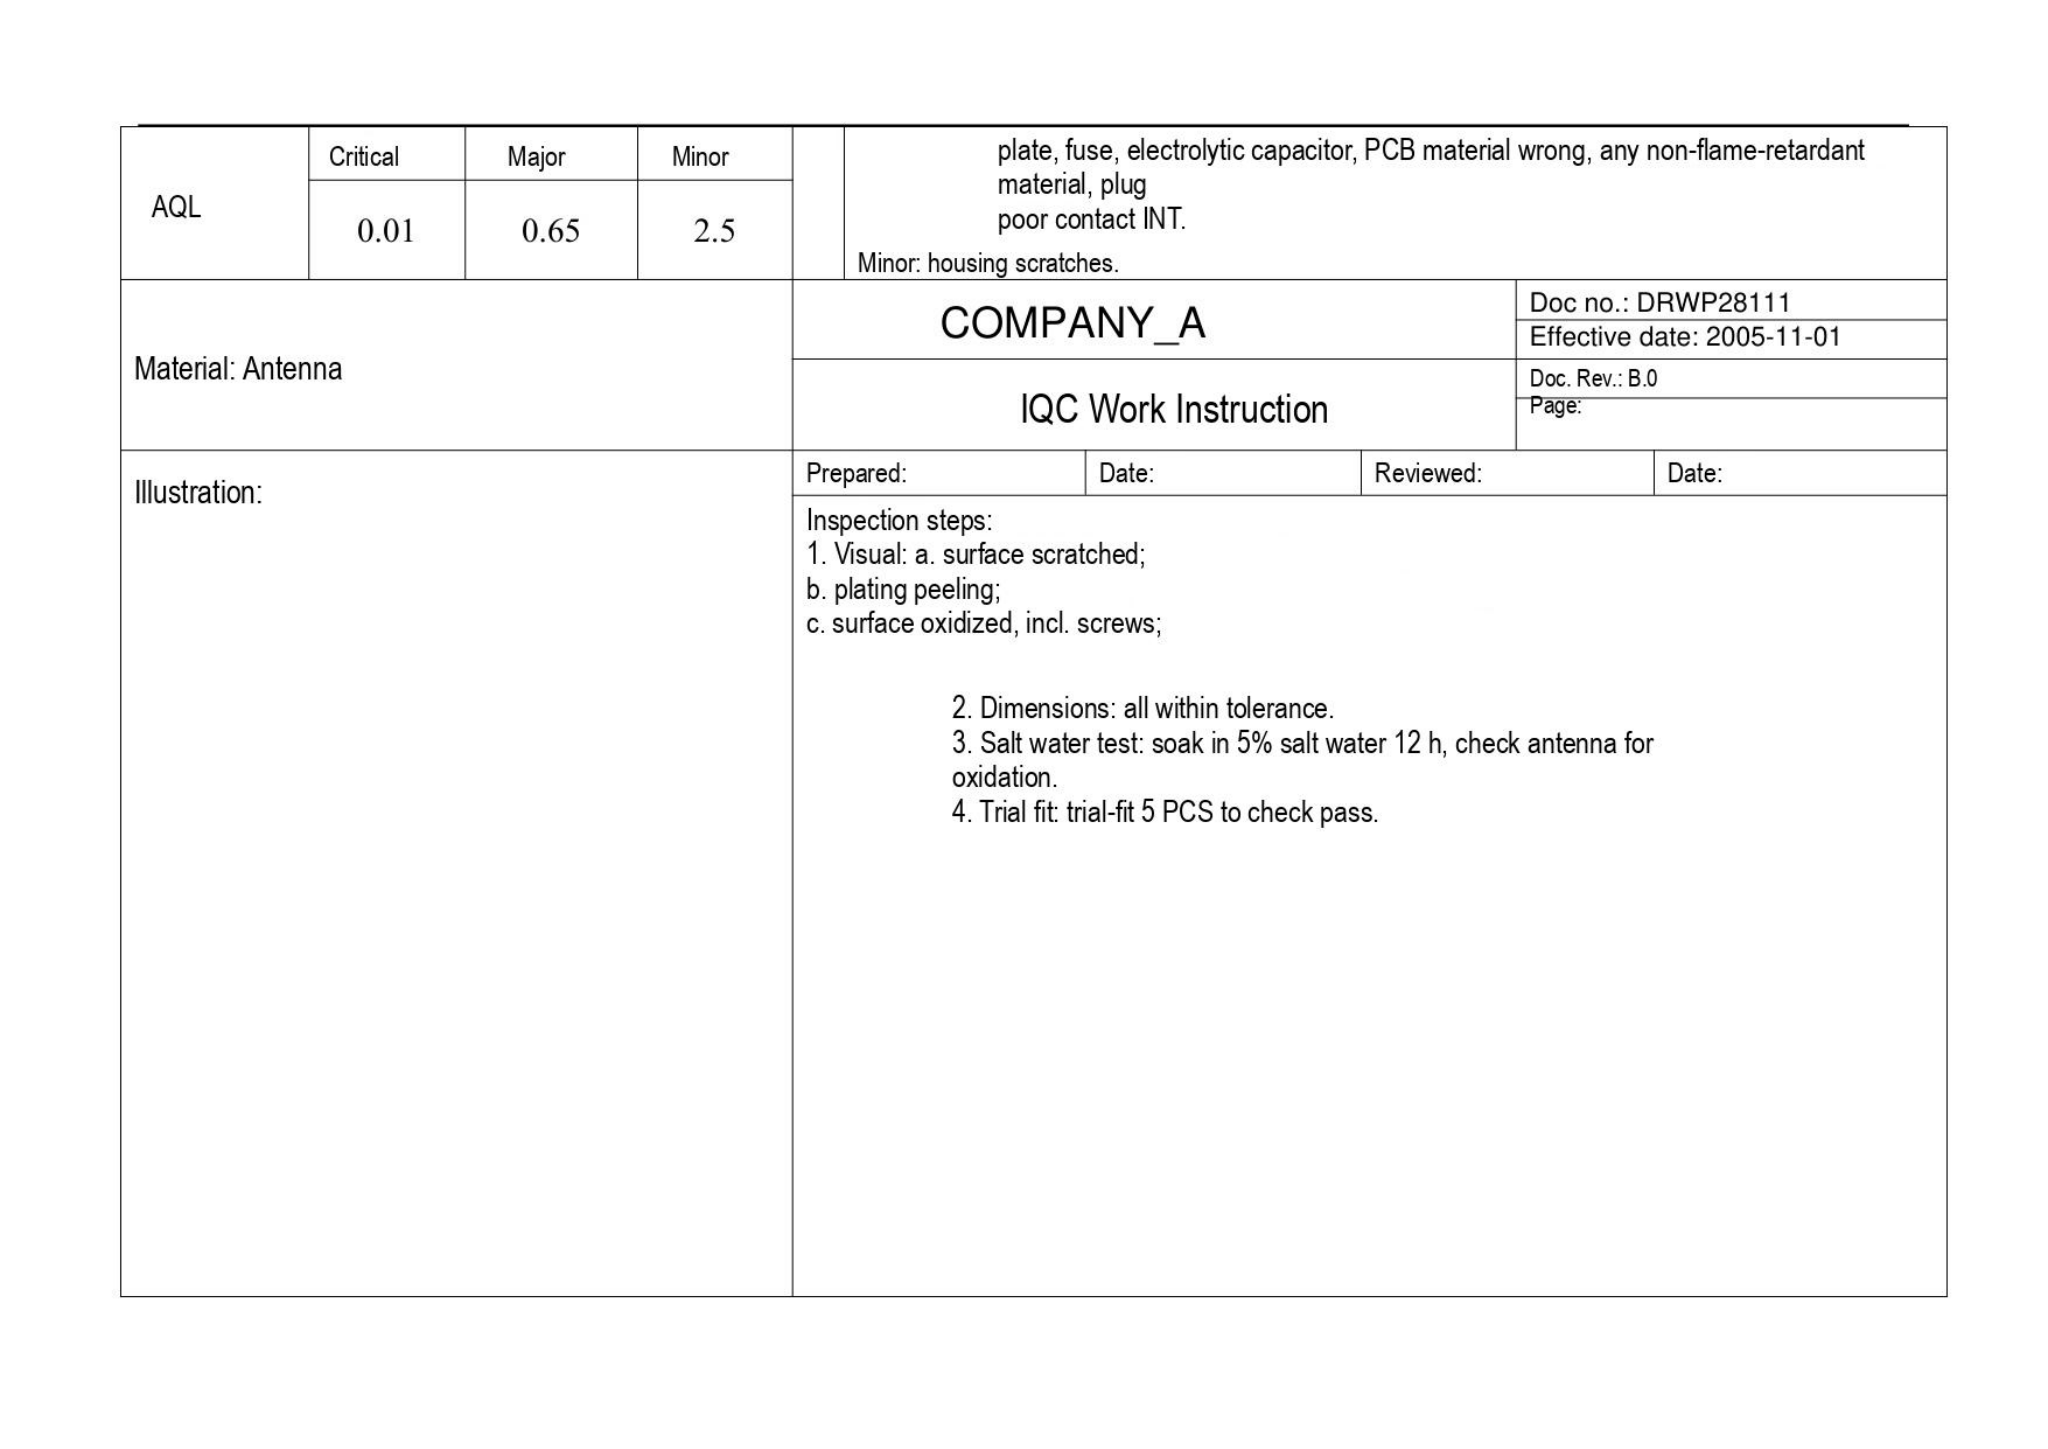| AQL | Critical | Major | Minor |
|---|---|---|---|
| | 0.01 | 0.65 | 2.5 |

plate, fuse, electrolytic capacitor, PCB material wrong, any non-flame-retardant material, plug
poor contact INT.
Minor: housing scratches.

Material: Antenna

| COMPANY_A | Doc no.: DRWP28111 |
|---|---|
| | Effective date: 2005-11-01 |
| IQC Work Instruction | Doc. Rev.: B.0 |
| | Page: |

Illustration:

| Prepared: | Date: | Reviewed: | Date: |
|---|---|---|---|

Inspection steps:
1. Visual: a. surface scratched;
b. plating peeling;
c. surface oxidized, incl. screws;

2. Dimensions: all within tolerance.
3. Salt water test: soak in 5% salt water 12 h, check antenna for oxidation.
4. Trial fit: trial-fit 5 PCS to check pass.
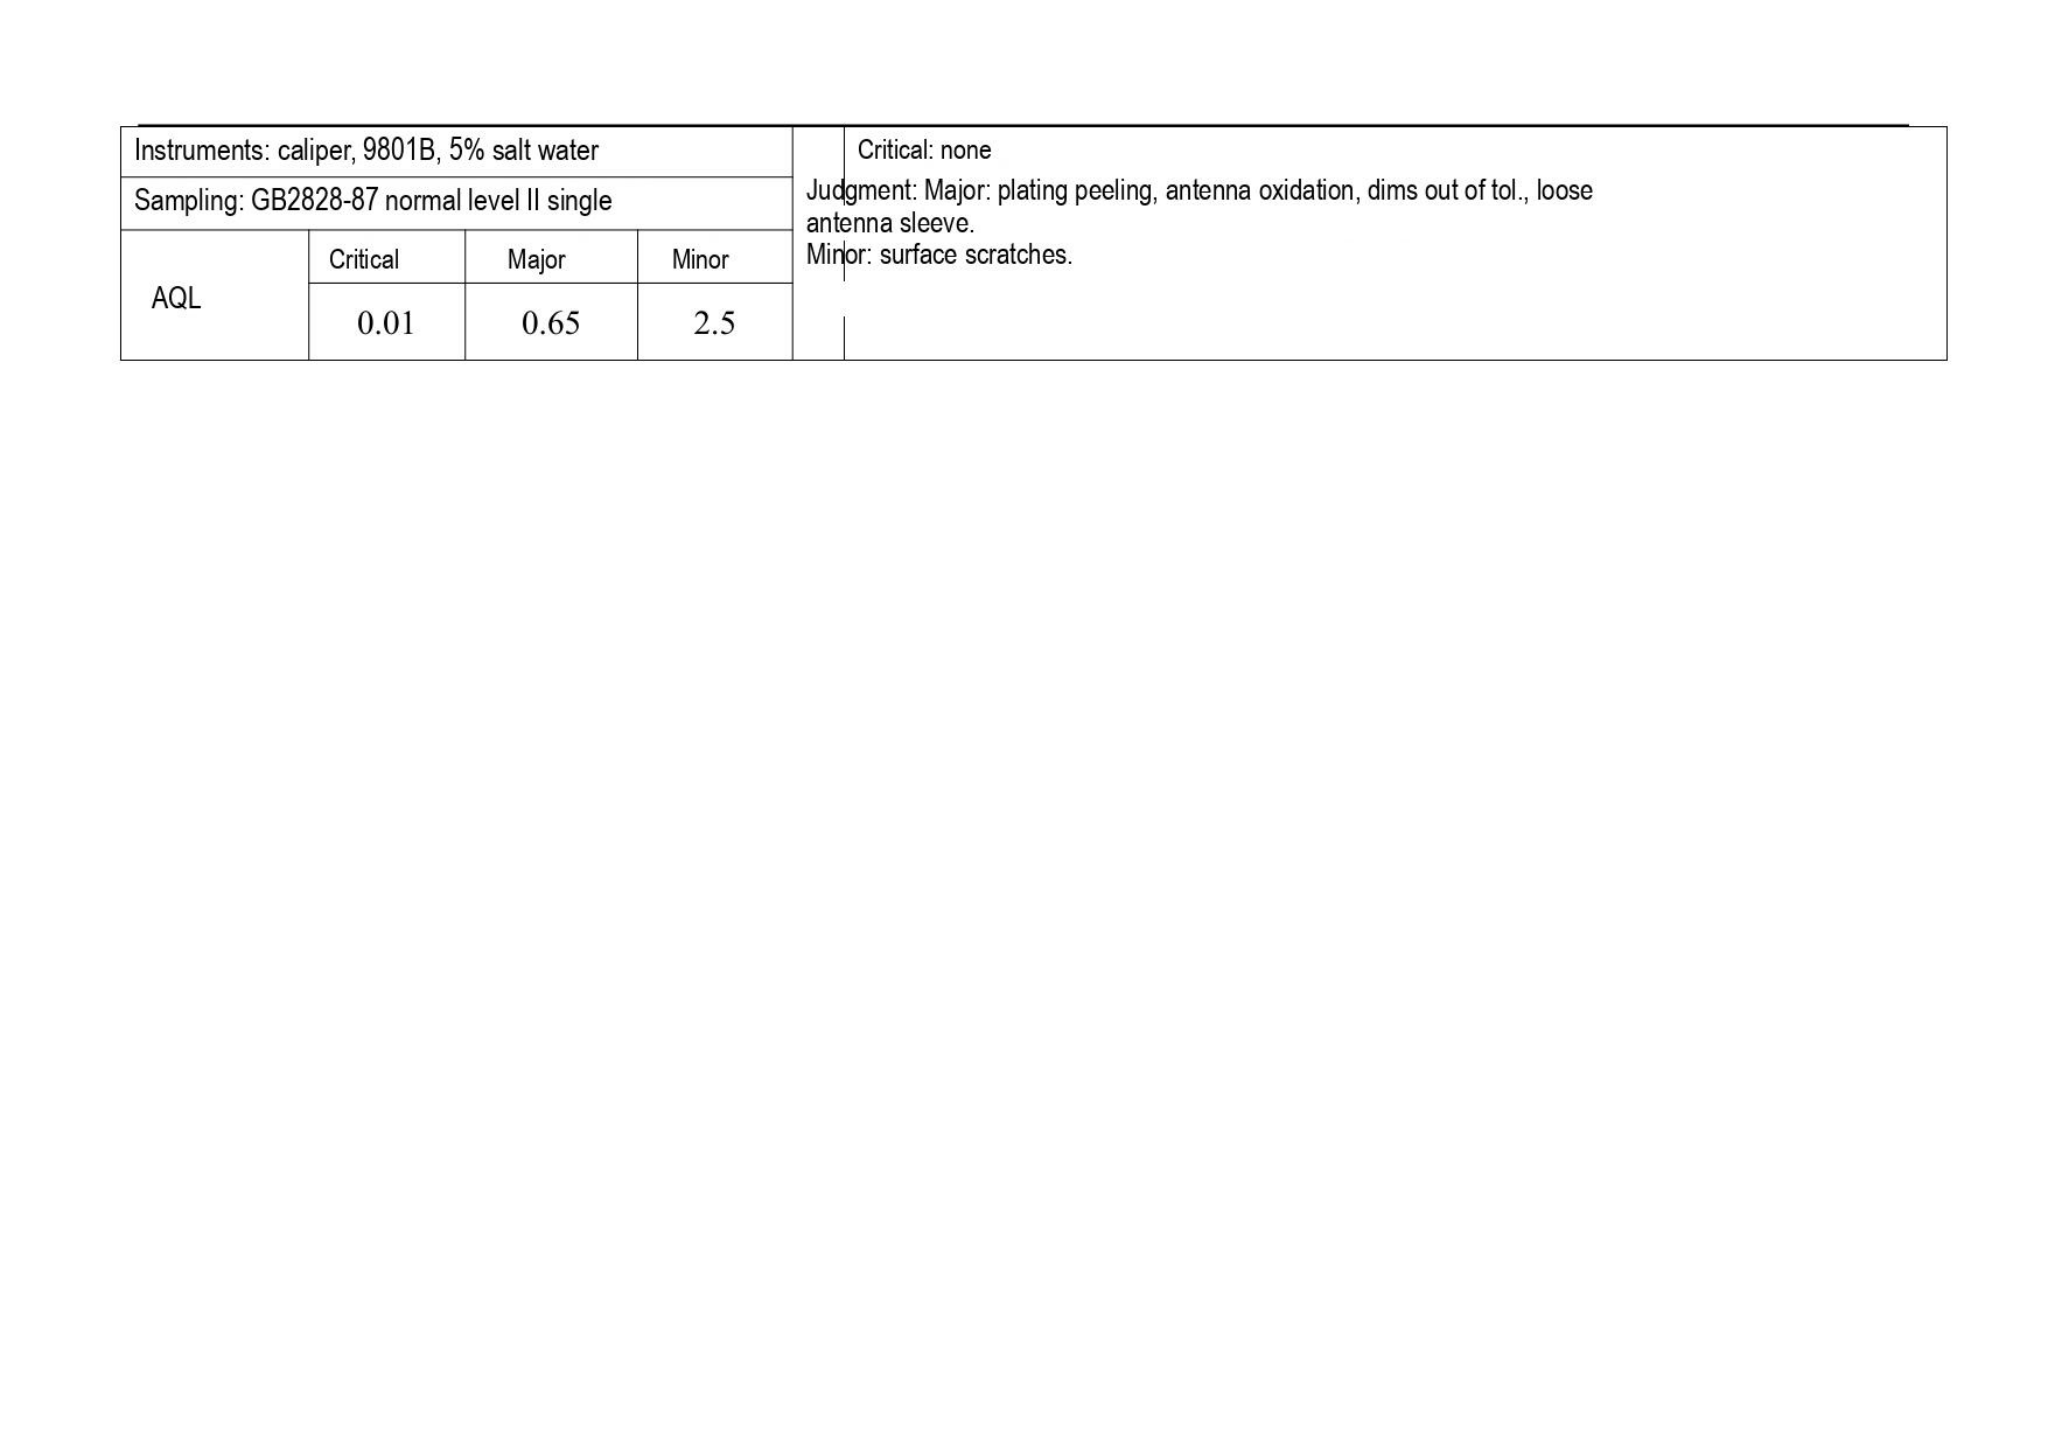| Instruments: caliper, 9801B, 5% salt water | | | | Critical: none<br>Judgment: Major: plating peeling, antenna oxidation, dims out of tol., loose antenna sleeve.<br>Minor: surface scratches. |
|---|---|---|---|---|
| Sampling: GB2828-87 normal level II single | | | | |
| AQL | Critical | Major | Minor | |
| | 0.01 | 0.65 | 2.5 | |